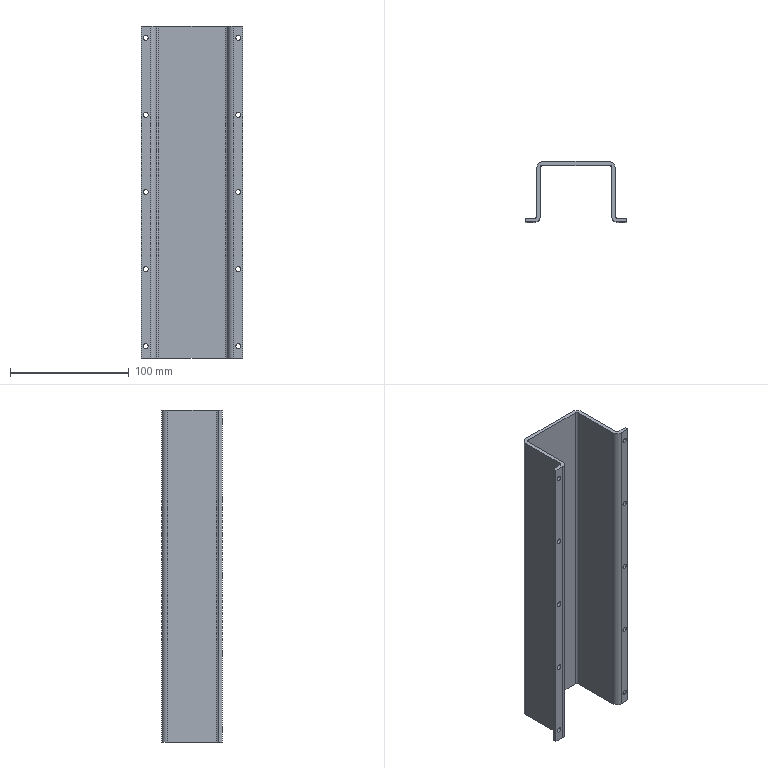Part | SolidWorks | features Extrusion 1, ICE 1, LPattern 1 | 1 solid | 42 faces | box 86 x 51 x 280 mm | volume 147456 mm3 | cylinder 28 | plane 14 | commonest cylinder face diameters 4 x24 10 x4
STEP:
#1=CARTESIAN_POINT('',(80.,3.,205.));
#2=VERTEX_POINT('',#1);
#3=CARTESIAN_POINT('',(84.,3.,205.));
#4=VERTEX_POINT('',#3);
#5=CARTESIAN_POINT('',(82.,3.,205.));
#6=DIRECTION('',(0.,-1.,0.));
#7=DIRECTION('',(1.,0.,0.));
#8=AXIS2_PLACEMENT_3D('',#5,#6,#7);
#9=CIRCLE('',#8,2.);
#10=EDGE_CURVE('',#2,#4,#9,.T.);
#11=ORIENTED_EDGE('',*,*,#10,.F.);
#12=CARTESIAN_POINT('',(80.,0.,205.));
#13=VERTEX_POINT('',#12);
#14=CARTESIAN_POINT('',(80.,10.,205.));
#15=DIRECTION('',(0.,-1.,0.));
#16=VECTOR('',#15,1000.);
#17=LINE('',#14,#16);
#18=EDGE_CURVE('',#2,#13,#17,.T.);
#19=ORIENTED_EDGE('',*,*,#18,.T.);
#20=CARTESIAN_POINT('',(84.,0.,205.));
#21=VERTEX_POINT('',#20);
#22=CARTESIAN_POINT('',(82.,0.,205.));
#23=DIRECTION('',(0.,-1.,0.));
#24=DIRECTION('',(1.,0.,0.));
#25=AXIS2_PLACEMENT_3D('',#22,#23,#24);
#26=CIRCLE('',#25,2.);
#27=EDGE_CURVE('',#13,#21,#26,.T.);
#28=ORIENTED_EDGE('',*,*,#27,.T.);
#29=CARTESIAN_POINT('',(84.,10.,205.));
#30=DIRECTION('',(0.,-1.,0.));
#31=VECTOR('',#30,1000.);
#32=LINE('',#29,#31);
#33=EDGE_CURVE('',#4,#21,#32,.T.);
#34=ORIENTED_EDGE('',*,*,#33,.F.);
#35=EDGE_LOOP('',(#11,#19,#28,#34));
#36=FACE_OUTER_BOUND('',#35,.T.);
#37=CARTESIAN_POINT('',(82.,10.,205.));
#38=DIRECTION('',(0.,-1.,0.));
#39=DIRECTION('',(1.,0.,0.));
#40=AXIS2_PLACEMENT_3D('',#37,#38,#39);
#41=CYLINDRICAL_SURFACE('',#40,2.);
#42=ADVANCED_FACE('',(#36),#41,.F.);
#43=CARTESIAN_POINT('',(80.,3.,140.));
#44=VERTEX_POINT('',#43);
#45=CARTESIAN_POINT('',(84.,3.,140.));
#46=VERTEX_POINT('',#45);
#47=CARTESIAN_POINT('',(82.,3.,140.));
#48=DIRECTION('',(0.,-1.,0.));
#49=DIRECTION('',(1.,0.,0.));
#50=AXIS2_PLACEMENT_3D('',#47,#48,#49);
#51=CIRCLE('',#50,2.);
#52=EDGE_CURVE('',#44,#46,#51,.T.);
#53=ORIENTED_EDGE('',*,*,#52,.F.);
#54=CARTESIAN_POINT('',(80.,0.,140.));
#55=VERTEX_POINT('',#54);
#56=CARTESIAN_POINT('',(80.,10.,140.));
#57=DIRECTION('',(0.,-1.,0.));
#58=VECTOR('',#57,1000.);
#59=LINE('',#56,#58);
#60=EDGE_CURVE('',#44,#55,#59,.T.);
#61=ORIENTED_EDGE('',*,*,#60,.T.);
#62=CARTESIAN_POINT('',(84.,0.,140.));
#63=VERTEX_POINT('',#62);
#64=CARTESIAN_POINT('',(82.,0.,140.));
#65=DIRECTION('',(0.,-1.,0.));
#66=DIRECTION('',(1.,0.,0.));
#67=AXIS2_PLACEMENT_3D('',#64,#65,#66);
#68=CIRCLE('',#67,2.);
#69=EDGE_CURVE('',#55,#63,#68,.T.);
#70=ORIENTED_EDGE('',*,*,#69,.T.);
#71=CARTESIAN_POINT('',(84.,10.,140.));
#72=DIRECTION('',(0.,-1.,0.));
#73=VECTOR('',#72,1000.);
#74=LINE('',#71,#73);
#75=EDGE_CURVE('',#46,#63,#74,.T.);
#76=ORIENTED_EDGE('',*,*,#75,.F.);
#77=EDGE_LOOP('',(#53,#61,#70,#76));
#78=FACE_OUTER_BOUND('',#77,.T.);
#79=CARTESIAN_POINT('',(82.,10.,140.));
#80=DIRECTION('',(0.,-1.,0.));
#81=DIRECTION('',(1.,0.,0.));
#82=AXIS2_PLACEMENT_3D('',#79,#80,#81);
#83=CYLINDRICAL_SURFACE('',#82,2.);
#84=ADVANCED_FACE('',(#78),#83,.F.);
#85=CARTESIAN_POINT('',(80.,3.,75.));
#86=VERTEX_POINT('',#85);
#87=CARTESIAN_POINT('',(84.,3.,75.));
#88=VERTEX_POINT('',#87);
#89=CARTESIAN_POINT('',(82.,3.,75.));
#90=DIRECTION('',(0.,-1.,0.));
#91=DIRECTION('',(1.,0.,0.));
#92=AXIS2_PLACEMENT_3D('',#89,#90,#91);
#93=CIRCLE('',#92,2.);
#94=EDGE_CURVE('',#86,#88,#93,.T.);
#95=ORIENTED_EDGE('',*,*,#94,.F.);
#96=CARTESIAN_POINT('',(80.,0.,75.));
#97=VERTEX_POINT('',#96);
#98=CARTESIAN_POINT('',(80.,10.,75.));
#99=DIRECTION('',(0.,-1.,0.));
#100=VECTOR('',#99,1000.);
#101=LINE('',#98,#100);
#102=EDGE_CURVE('',#86,#97,#101,.T.);
#103=ORIENTED_EDGE('',*,*,#102,.T.);
#104=CARTESIAN_POINT('',(84.,0.,75.));
#105=VERTEX_POINT('',#104);
#106=CARTESIAN_POINT('',(82.,0.,75.));
#107=DIRECTION('',(0.,-1.,0.));
#108=DIRECTION('',(1.,0.,0.));
#109=AXIS2_PLACEMENT_3D('',#106,#107,#108);
#110=CIRCLE('',#109,2.);
#111=EDGE_CURVE('',#97,#105,#110,.T.);
#112=ORIENTED_EDGE('',*,*,#111,.T.);
#113=CARTESIAN_POINT('',(84.,10.,75.));
#114=DIRECTION('',(0.,-1.,0.));
#115=VECTOR('',#114,1000.);
#116=LINE('',#113,#115);
#117=EDGE_CURVE('',#88,#105,#116,.T.);
#118=ORIENTED_EDGE('',*,*,#117,.F.);
#119=EDGE_LOOP('',(#95,#103,#112,#118));
#120=FACE_OUTER_BOUND('',#119,.T.);
#121=CARTESIAN_POINT('',(82.,10.,75.));
#122=DIRECTION('',(0.,-1.,0.));
#123=DIRECTION('',(1.,0.,0.));
#124=AXIS2_PLACEMENT_3D('',#121,#122,#123);
#125=CYLINDRICAL_SURFACE('',#124,2.);
#126=ADVANCED_FACE('',(#120),#125,.F.);
#127=CARTESIAN_POINT('',(80.,3.,10.));
#128=VERTEX_POINT('',#127);
#129=CARTESIAN_POINT('',(84.,3.,10.));
#130=VERTEX_POINT('',#129);
#131=CARTESIAN_POINT('',(82.,3.,10.));
#132=DIRECTION('',(0.,-1.,0.));
#133=DIRECTION('',(1.,0.,0.));
#134=AXIS2_PLACEMENT_3D('',#131,#132,#133);
#135=CIRCLE('',#134,2.);
#136=EDGE_CURVE('',#128,#130,#135,.T.);
#137=ORIENTED_EDGE('',*,*,#136,.F.);
#138=CARTESIAN_POINT('',(80.,0.,10.));
#139=VERTEX_POINT('',#138);
#140=CARTESIAN_POINT('',(80.,10.,10.));
#141=DIRECTION('',(0.,-1.,0.));
#142=VECTOR('',#141,1000.);
#143=LINE('',#140,#142);
#144=EDGE_CURVE('',#128,#139,#143,.T.);
#145=ORIENTED_EDGE('',*,*,#144,.T.);
#146=CARTESIAN_POINT('',(84.,0.,10.));
#147=VERTEX_POINT('',#146);
#148=CARTESIAN_POINT('',(82.,0.,10.));
#149=DIRECTION('',(0.,-1.,0.));
#150=DIRECTION('',(1.,0.,0.));
#151=AXIS2_PLACEMENT_3D('',#148,#149,#150);
#152=CIRCLE('',#151,2.);
#153=EDGE_CURVE('',#139,#147,#152,.T.);
#154=ORIENTED_EDGE('',*,*,#153,.T.);
#155=CARTESIAN_POINT('',(84.,10.,10.));
#156=DIRECTION('',(0.,-1.,0.));
#157=VECTOR('',#156,1000.);
#158=LINE('',#155,#157);
#159=EDGE_CURVE('',#130,#147,#158,.T.);
#160=ORIENTED_EDGE('',*,*,#159,.F.);
#161=EDGE_LOOP('',(#137,#145,#154,#160));
#162=FACE_OUTER_BOUND('',#161,.T.);
#163=CARTESIAN_POINT('',(82.,10.,10.));
#164=DIRECTION('',(0.,-1.,0.));
#165=DIRECTION('',(1.,0.,0.));
#166=AXIS2_PLACEMENT_3D('',#163,#164,#165);
#167=CYLINDRICAL_SURFACE('',#166,2.);
#168=ADVANCED_FACE('',(#162),#167,.F.);
#169=CARTESIAN_POINT('',(2.,3.,140.));
#170=VERTEX_POINT('',#169);
#171=CARTESIAN_POINT('',(6.,3.,140.));
#172=VERTEX_POINT('',#171);
#173=CARTESIAN_POINT('',(4.,3.,140.));
#174=DIRECTION('',(0.,-1.,0.));
#175=DIRECTION('',(0.,0.,-1.));
#176=AXIS2_PLACEMENT_3D('',#173,#174,#175);
#177=CIRCLE('',#176,2.);
#178=EDGE_CURVE('',#170,#172,#177,.T.);
#179=ORIENTED_EDGE('',*,*,#178,.F.);
#180=CARTESIAN_POINT('',(2.,0.,140.));
#181=VERTEX_POINT('',#180);
#182=CARTESIAN_POINT('',(2.,10.,140.));
#183=DIRECTION('',(0.,-1.,0.));
#184=VECTOR('',#183,1000.);
#185=LINE('',#182,#184);
#186=EDGE_CURVE('',#170,#181,#185,.T.);
#187=ORIENTED_EDGE('',*,*,#186,.T.);
#188=CARTESIAN_POINT('',(6.,0.,140.));
#189=VERTEX_POINT('',#188);
#190=CARTESIAN_POINT('',(4.,0.,140.));
#191=DIRECTION('',(0.,-1.,0.));
#192=DIRECTION('',(1.,0.,0.));
#193=AXIS2_PLACEMENT_3D('',#190,#191,#192);
#194=CIRCLE('',#193,2.);
#195=EDGE_CURVE('',#181,#189,#194,.T.);
#196=ORIENTED_EDGE('',*,*,#195,.T.);
#197=CARTESIAN_POINT('',(6.,10.,140.));
#198=DIRECTION('',(0.,-1.,0.));
#199=VECTOR('',#198,1000.);
#200=LINE('',#197,#199);
#201=EDGE_CURVE('',#172,#189,#200,.T.);
#202=ORIENTED_EDGE('',*,*,#201,.F.);
#203=EDGE_LOOP('',(#179,#187,#196,#202));
#204=FACE_OUTER_BOUND('',#203,.T.);
#205=CARTESIAN_POINT('',(4.,10.,140.));
#206=DIRECTION('',(0.,-1.,0.));
#207=DIRECTION('',(1.,0.,0.));
#208=AXIS2_PLACEMENT_3D('',#205,#206,#207);
#209=CYLINDRICAL_SURFACE('',#208,2.);
#210=ADVANCED_FACE('',(#204),#209,.F.);
#211=CARTESIAN_POINT('',(2.,3.,75.));
#212=VERTEX_POINT('',#211);
#213=CARTESIAN_POINT('',(6.,3.,75.));
#214=VERTEX_POINT('',#213);
#215=CARTESIAN_POINT('',(4.,3.,75.));
#216=DIRECTION('',(0.,-1.,0.));
#217=DIRECTION('',(0.,0.,-1.));
#218=AXIS2_PLACEMENT_3D('',#215,#216,#217);
#219=CIRCLE('',#218,2.);
#220=EDGE_CURVE('',#212,#214,#219,.T.);
#221=ORIENTED_EDGE('',*,*,#220,.F.);
#222=CARTESIAN_POINT('',(2.,0.,75.));
#223=VERTEX_POINT('',#222);
#224=CARTESIAN_POINT('',(2.,10.,75.));
#225=DIRECTION('',(0.,-1.,0.));
#226=VECTOR('',#225,1000.);
#227=LINE('',#224,#226);
#228=EDGE_CURVE('',#212,#223,#227,.T.);
#229=ORIENTED_EDGE('',*,*,#228,.T.);
#230=CARTESIAN_POINT('',(6.,0.,75.));
#231=VERTEX_POINT('',#230);
#232=CARTESIAN_POINT('',(4.,0.,75.));
#233=DIRECTION('',(0.,-1.,0.));
#234=DIRECTION('',(1.,0.,0.));
#235=AXIS2_PLACEMENT_3D('',#232,#233,#234);
#236=CIRCLE('',#235,2.);
#237=EDGE_CURVE('',#223,#231,#236,.T.);
#238=ORIENTED_EDGE('',*,*,#237,.T.);
#239=CARTESIAN_POINT('',(6.,10.,75.));
#240=DIRECTION('',(0.,-1.,0.));
#241=VECTOR('',#240,1000.);
#242=LINE('',#239,#241);
#243=EDGE_CURVE('',#214,#231,#242,.T.);
#244=ORIENTED_EDGE('',*,*,#243,.F.);
#245=EDGE_LOOP('',(#221,#229,#238,#244));
#246=FACE_OUTER_BOUND('',#245,.T.);
#247=CARTESIAN_POINT('',(4.,10.,75.));
#248=DIRECTION('',(0.,-1.,0.));
#249=DIRECTION('',(1.,0.,0.));
#250=AXIS2_PLACEMENT_3D('',#247,#248,#249);
#251=CYLINDRICAL_SURFACE('',#250,2.);
#252=ADVANCED_FACE('',(#246),#251,.F.);
#253=CARTESIAN_POINT('',(2.,3.,10.));
#254=VERTEX_POINT('',#253);
#255=CARTESIAN_POINT('',(6.,3.,10.));
#256=VERTEX_POINT('',#255);
#257=CARTESIAN_POINT('',(4.,3.,10.));
#258=DIRECTION('',(0.,-1.,0.));
#259=DIRECTION('',(0.,0.,-1.));
#260=AXIS2_PLACEMENT_3D('',#257,#258,#259);
#261=CIRCLE('',#260,2.);
#262=EDGE_CURVE('',#254,#256,#261,.T.);
#263=ORIENTED_EDGE('',*,*,#262,.F.);
#264=CARTESIAN_POINT('',(2.,0.,10.));
#265=VERTEX_POINT('',#264);
#266=CARTESIAN_POINT('',(2.,10.,10.));
#267=DIRECTION('',(0.,-1.,0.));
#268=VECTOR('',#267,1000.);
#269=LINE('',#266,#268);
#270=EDGE_CURVE('',#254,#265,#269,.T.);
#271=ORIENTED_EDGE('',*,*,#270,.T.);
#272=CARTESIAN_POINT('',(6.,0.,10.));
#273=VERTEX_POINT('',#272);
#274=CARTESIAN_POINT('',(4.,0.,10.));
#275=DIRECTION('',(0.,-1.,0.));
#276=DIRECTION('',(1.,0.,0.));
#277=AXIS2_PLACEMENT_3D('',#274,#275,#276);
#278=CIRCLE('',#277,2.);
#279=EDGE_CURVE('',#265,#273,#278,.T.);
#280=ORIENTED_EDGE('',*,*,#279,.T.);
#281=CARTESIAN_POINT('',(6.,10.,10.));
#282=DIRECTION('',(0.,-1.,0.));
#283=VECTOR('',#282,1000.);
#284=LINE('',#281,#283);
#285=EDGE_CURVE('',#256,#273,#284,.T.);
#286=ORIENTED_EDGE('',*,*,#285,.F.);
#287=EDGE_LOOP('',(#263,#271,#280,#286));
#288=FACE_OUTER_BOUND('',#287,.T.);
#289=CARTESIAN_POINT('',(4.,10.,10.));
#290=DIRECTION('',(0.,-1.,0.));
#291=DIRECTION('',(1.,0.,0.));
#292=AXIS2_PLACEMENT_3D('',#289,#290,#291);
#293=CYLINDRICAL_SURFACE('',#292,2.);
#294=ADVANCED_FACE('',(#288),#293,.F.);
#295=CARTESIAN_POINT('',(2.,3.,205.));
#296=VERTEX_POINT('',#295);
#297=CARTESIAN_POINT('',(6.,3.,205.));
#298=VERTEX_POINT('',#297);
#299=CARTESIAN_POINT('',(4.,3.,205.));
#300=DIRECTION('',(0.,-1.,0.));
#301=DIRECTION('',(0.,0.,-1.));
#302=AXIS2_PLACEMENT_3D('',#299,#300,#301);
#303=CIRCLE('',#302,2.);
#304=EDGE_CURVE('',#296,#298,#303,.T.);
#305=ORIENTED_EDGE('',*,*,#304,.F.);
#306=CARTESIAN_POINT('',(2.,0.,205.));
#307=VERTEX_POINT('',#306);
#308=CARTESIAN_POINT('',(2.,10.,205.));
#309=DIRECTION('',(0.,-1.,0.));
#310=VECTOR('',#309,1000.);
#311=LINE('',#308,#310);
#312=EDGE_CURVE('',#296,#307,#311,.T.);
#313=ORIENTED_EDGE('',*,*,#312,.T.);
#314=CARTESIAN_POINT('',(6.,0.,205.));
#315=VERTEX_POINT('',#314);
#316=CARTESIAN_POINT('',(4.,0.,205.));
#317=DIRECTION('',(0.,-1.,0.));
#318=DIRECTION('',(1.,0.,0.));
#319=AXIS2_PLACEMENT_3D('',#316,#317,#318);
#320=CIRCLE('',#319,2.);
#321=EDGE_CURVE('',#307,#315,#320,.T.);
#322=ORIENTED_EDGE('',*,*,#321,.T.);
#323=CARTESIAN_POINT('',(6.,10.,205.));
#324=DIRECTION('',(0.,-1.,0.));
#325=VECTOR('',#324,1000.);
#326=LINE('',#323,#325);
#327=EDGE_CURVE('',#298,#315,#326,.T.);
#328=ORIENTED_EDGE('',*,*,#327,.F.);
#329=EDGE_LOOP('',(#305,#313,#322,#328));
#330=FACE_OUTER_BOUND('',#329,.T.);
#331=CARTESIAN_POINT('',(4.,10.,205.));
#332=DIRECTION('',(0.,-1.,0.));
#333=DIRECTION('',(1.,0.,0.));
#334=AXIS2_PLACEMENT_3D('',#331,#332,#333);
#335=CYLINDRICAL_SURFACE('',#334,2.);
#336=ADVANCED_FACE('',(#330),#335,.F.);
#337=CARTESIAN_POINT('',(80.,3.,270.));
#338=VERTEX_POINT('',#337);
#339=CARTESIAN_POINT('',(84.,3.,270.));
#340=VERTEX_POINT('',#339);
#341=CARTESIAN_POINT('',(82.,3.,270.));
#342=DIRECTION('',(0.,-1.,0.));
#343=DIRECTION('',(1.,0.,0.));
#344=AXIS2_PLACEMENT_3D('',#341,#342,#343);
#345=CIRCLE('',#344,2.);
#346=EDGE_CURVE('',#338,#340,#345,.T.);
#347=ORIENTED_EDGE('',*,*,#346,.F.);
#348=CARTESIAN_POINT('',(80.,0.,270.));
#349=VERTEX_POINT('',#348);
#350=CARTESIAN_POINT('',(80.,10.,270.));
#351=DIRECTION('',(0.,-1.,0.));
#352=VECTOR('',#351,1000.);
#353=LINE('',#350,#352);
#354=EDGE_CURVE('',#338,#349,#353,.T.);
#355=ORIENTED_EDGE('',*,*,#354,.T.);
#356=CARTESIAN_POINT('',(84.,0.,270.));
#357=VERTEX_POINT('',#356);
#358=CARTESIAN_POINT('',(82.,0.,270.));
#359=DIRECTION('',(0.,-1.,0.));
#360=DIRECTION('',(1.,0.,0.));
#361=AXIS2_PLACEMENT_3D('',#358,#359,#360);
#362=CIRCLE('',#361,2.);
#363=EDGE_CURVE('',#349,#357,#362,.T.);
#364=ORIENTED_EDGE('',*,*,#363,.T.);
#365=CARTESIAN_POINT('',(84.,10.,270.));
#366=DIRECTION('',(0.,-1.,0.));
#367=VECTOR('',#366,1000.);
#368=LINE('',#365,#367);
#369=EDGE_CURVE('',#340,#357,#368,.T.);
#370=ORIENTED_EDGE('',*,*,#369,.F.);
#371=EDGE_LOOP('',(#347,#355,#364,#370));
#372=FACE_OUTER_BOUND('',#371,.T.);
#373=CARTESIAN_POINT('',(82.,10.,270.));
#374=DIRECTION('',(0.,-1.,0.));
#375=DIRECTION('',(1.,0.,0.));
#376=AXIS2_PLACEMENT_3D('',#373,#374,#375);
#377=CYLINDRICAL_SURFACE('',#376,2.);
#378=ADVANCED_FACE('',(#372),#377,.F.);
#379=CARTESIAN_POINT('',(2.,3.,270.));
#380=VERTEX_POINT('',#379);
#381=CARTESIAN_POINT('',(6.,3.,270.));
#382=VERTEX_POINT('',#381);
#383=CARTESIAN_POINT('',(4.,3.,270.));
#384=DIRECTION('',(0.,-1.,0.));
#385=DIRECTION('',(0.,0.,-1.));
#386=AXIS2_PLACEMENT_3D('',#383,#384,#385);
#387=CIRCLE('',#386,2.);
#388=EDGE_CURVE('',#380,#382,#387,.T.);
#389=ORIENTED_EDGE('',*,*,#388,.F.);
#390=CARTESIAN_POINT('',(2.,0.,270.));
#391=VERTEX_POINT('',#390);
#392=CARTESIAN_POINT('',(2.,10.,270.));
#393=DIRECTION('',(0.,-1.,0.));
#394=VECTOR('',#393,1000.);
#395=LINE('',#392,#394);
#396=EDGE_CURVE('',#380,#391,#395,.T.);
#397=ORIENTED_EDGE('',*,*,#396,.T.);
#398=CARTESIAN_POINT('',(6.,0.,270.));
#399=VERTEX_POINT('',#398);
#400=CARTESIAN_POINT('',(4.,0.,270.));
#401=DIRECTION('',(0.,-1.,0.));
#402=DIRECTION('',(1.,0.,0.));
#403=AXIS2_PLACEMENT_3D('',#400,#401,#402);
#404=CIRCLE('',#403,2.);
#405=EDGE_CURVE('',#391,#399,#404,.T.);
#406=ORIENTED_EDGE('',*,*,#405,.T.);
#407=CARTESIAN_POINT('',(6.,10.,270.));
#408=DIRECTION('',(0.,-1.,0.));
#409=VECTOR('',#408,1000.);
#410=LINE('',#407,#409);
#411=EDGE_CURVE('',#382,#399,#410,.T.);
#412=ORIENTED_EDGE('',*,*,#411,.F.);
#413=EDGE_LOOP('',(#389,#397,#406,#412));
#414=FACE_OUTER_BOUND('',#413,.T.);
#415=CARTESIAN_POINT('',(4.,10.,270.));
#416=DIRECTION('',(0.,-1.,0.));
#417=DIRECTION('',(1.,0.,0.));
#418=AXIS2_PLACEMENT_3D('',#415,#416,#417);
#419=CYLINDRICAL_SURFACE('',#418,2.);
#420=ADVANCED_FACE('',(#414),#419,.F.);
#421=CARTESIAN_POINT('',(4.,0.,140.));
#422=DIRECTION('',(0.,-1.,0.));
#423=DIRECTION('',(1.,0.,0.));
#424=AXIS2_PLACEMENT_3D('',#421,#422,#423);
#425=CIRCLE('',#424,2.);
#426=EDGE_CURVE('',#189,#181,#425,.T.);
#427=ORIENTED_EDGE('',*,*,#426,.F.);
#428=ORIENTED_EDGE('',*,*,#195,.F.);
#429=EDGE_LOOP('',(#427,#428));
#430=FACE_BOUND('',#429,.T.);
#431=CARTESIAN_POINT('',(4.,0.,75.));
#432=DIRECTION('',(0.,-1.,0.));
#433=DIRECTION('',(1.,0.,0.));
#434=AXIS2_PLACEMENT_3D('',#431,#432,#433);
#435=CIRCLE('',#434,2.);
#436=EDGE_CURVE('',#231,#223,#435,.T.);
#437=ORIENTED_EDGE('',*,*,#436,.F.);
#438=ORIENTED_EDGE('',*,*,#237,.F.);
#439=EDGE_LOOP('',(#437,#438));
#440=FACE_BOUND('',#439,.T.);
#441=CARTESIAN_POINT('',(4.,0.,10.));
#442=DIRECTION('',(0.,-1.,0.));
#443=DIRECTION('',(1.,0.,0.));
#444=AXIS2_PLACEMENT_3D('',#441,#442,#443);
#445=CIRCLE('',#444,2.);
#446=EDGE_CURVE('',#273,#265,#445,.T.);
#447=ORIENTED_EDGE('',*,*,#446,.F.);
#448=ORIENTED_EDGE('',*,*,#279,.F.);
#449=EDGE_LOOP('',(#447,#448));
#450=FACE_BOUND('',#449,.T.);
#451=CARTESIAN_POINT('',(4.,0.,205.));
#452=DIRECTION('',(0.,-1.,0.));
#453=DIRECTION('',(1.,0.,0.));
#454=AXIS2_PLACEMENT_3D('',#451,#452,#453);
#455=CIRCLE('',#454,2.);
#456=EDGE_CURVE('',#315,#307,#455,.T.);
#457=ORIENTED_EDGE('',*,*,#456,.F.);
#458=ORIENTED_EDGE('',*,*,#321,.F.);
#459=EDGE_LOOP('',(#457,#458));
#460=FACE_BOUND('',#459,.T.);
#461=CARTESIAN_POINT('',(4.,0.,270.));
#462=DIRECTION('',(0.,-1.,0.));
#463=DIRECTION('',(1.,0.,0.));
#464=AXIS2_PLACEMENT_3D('',#461,#462,#463);
#465=CIRCLE('',#464,2.);
#466=EDGE_CURVE('',#399,#391,#465,.T.);
#467=ORIENTED_EDGE('',*,*,#466,.F.);
#468=ORIENTED_EDGE('',*,*,#405,.F.);
#469=EDGE_LOOP('',(#467,#468));
#470=FACE_BOUND('',#469,.T.);
#471=CARTESIAN_POINT('',(0.,0.,0.));
#472=VERTEX_POINT('',#471);
#473=CARTESIAN_POINT('',(8.,0.,0.));
#474=VERTEX_POINT('',#473);
#475=CARTESIAN_POINT('',(8.,0.,0.));
#476=DIRECTION('',(1.,0.,0.));
#477=VECTOR('',#476,1000.);
#478=LINE('',#475,#477);
#479=EDGE_CURVE('',#472,#474,#478,.T.);
#480=ORIENTED_EDGE('',*,*,#479,.T.);
#481=CARTESIAN_POINT('',(8.,0.,280.));
#482=VERTEX_POINT('',#481);
#483=CARTESIAN_POINT('',(8.,0.,280.));
#484=DIRECTION('',(0.,0.,-1.));
#485=VECTOR('',#484,1000.);
#486=LINE('',#483,#485);
#487=EDGE_CURVE('',#482,#474,#486,.T.);
#488=ORIENTED_EDGE('',*,*,#487,.F.);
#489=CARTESIAN_POINT('',(0.,0.,280.));
#490=VERTEX_POINT('',#489);
#491=CARTESIAN_POINT('',(8.,0.,280.));
#492=DIRECTION('',(1.,0.,0.));
#493=VECTOR('',#492,1000.);
#494=LINE('',#491,#493);
#495=EDGE_CURVE('',#490,#482,#494,.T.);
#496=ORIENTED_EDGE('',*,*,#495,.F.);
#497=CARTESIAN_POINT('',(0.,0.,280.));
#498=DIRECTION('',(0.,0.,-1.));
#499=VECTOR('',#498,1000.);
#500=LINE('',#497,#499);
#501=EDGE_CURVE('',#490,#472,#500,.T.);
#502=ORIENTED_EDGE('',*,*,#501,.T.);
#503=EDGE_LOOP('',(#480,#488,#496,#502));
#504=FACE_OUTER_BOUND('',#503,.T.);
#505=CARTESIAN_POINT('',(8.,0.,280.));
#506=DIRECTION('',(0.,1.,0.));
#507=DIRECTION('',(-1.,0.,0.));
#508=AXIS2_PLACEMENT_3D('',#505,#506,#507);
#509=PLANE('',#508);
#510=ADVANCED_FACE('',(#430,#440,#450,#460,#470,#504),#509,.F.);
#511=CARTESIAN_POINT('',(13.,5.,0.));
#512=VERTEX_POINT('',#511);
#513=CARTESIAN_POINT('',(8.,5.,0.));
#514=DIRECTION('',(0.,0.,1.));
#515=DIRECTION('',(-1.,0.,0.));
#516=AXIS2_PLACEMENT_3D('',#513,#514,#515);
#517=CIRCLE('',#516,5.);
#518=EDGE_CURVE('',#474,#512,#517,.T.);
#519=ORIENTED_EDGE('',*,*,#518,.T.);
#520=CARTESIAN_POINT('',(13.,5.,280.));
#521=VERTEX_POINT('',#520);
#522=CARTESIAN_POINT('',(13.,5.,280.));
#523=DIRECTION('',(0.,0.,-1.));
#524=VECTOR('',#523,1000.);
#525=LINE('',#522,#524);
#526=EDGE_CURVE('',#521,#512,#525,.T.);
#527=ORIENTED_EDGE('',*,*,#526,.F.);
#528=CARTESIAN_POINT('',(8.,5.,280.));
#529=DIRECTION('',(0.,0.,1.));
#530=DIRECTION('',(-1.,0.,0.));
#531=AXIS2_PLACEMENT_3D('',#528,#529,#530);
#532=CIRCLE('',#531,5.);
#533=EDGE_CURVE('',#482,#521,#532,.T.);
#534=ORIENTED_EDGE('',*,*,#533,.F.);
#535=ORIENTED_EDGE('',*,*,#487,.T.);
#536=EDGE_LOOP('',(#519,#527,#534,#535));
#537=FACE_OUTER_BOUND('',#536,.T.);
#538=CARTESIAN_POINT('',(8.,5.,280.));
#539=DIRECTION('',(0.,0.,-1.));
#540=DIRECTION('',(-1.,0.,0.));
#541=AXIS2_PLACEMENT_3D('',#538,#539,#540);
#542=CYLINDRICAL_SURFACE('',#541,5.);
#543=ADVANCED_FACE('',(#537),#542,.T.);
#544=CARTESIAN_POINT('',(13.,46.,0.));
#545=VERTEX_POINT('',#544);
#546=CARTESIAN_POINT('',(13.,46.,0.));
#547=DIRECTION('',(0.,1.,0.));
#548=VECTOR('',#547,1000.);
#549=LINE('',#546,#548);
#550=EDGE_CURVE('',#512,#545,#549,.T.);
#551=ORIENTED_EDGE('',*,*,#550,.T.);
#552=CARTESIAN_POINT('',(13.,46.,280.));
#553=VERTEX_POINT('',#552);
#554=CARTESIAN_POINT('',(13.,46.,280.));
#555=DIRECTION('',(0.,0.,-1.));
#556=VECTOR('',#555,1000.);
#557=LINE('',#554,#556);
#558=EDGE_CURVE('',#553,#545,#557,.T.);
#559=ORIENTED_EDGE('',*,*,#558,.F.);
#560=CARTESIAN_POINT('',(13.,46.,280.));
#561=DIRECTION('',(0.,1.,0.));
#562=VECTOR('',#561,1000.);
#563=LINE('',#560,#562);
#564=EDGE_CURVE('',#521,#553,#563,.T.);
#565=ORIENTED_EDGE('',*,*,#564,.F.);
#566=ORIENTED_EDGE('',*,*,#526,.T.);
#567=EDGE_LOOP('',(#551,#559,#565,#566));
#568=FACE_OUTER_BOUND('',#567,.T.);
#569=CARTESIAN_POINT('',(13.,46.,280.));
#570=DIRECTION('',(-1.,0.,0.));
#571=DIRECTION('',(0.,0.,1.));
#572=AXIS2_PLACEMENT_3D('',#569,#570,#571);
#573=PLANE('',#572);
#574=ADVANCED_FACE('',(#568),#573,.F.);
#575=CARTESIAN_POINT('',(15.,48.,0.));
#576=VERTEX_POINT('',#575);
#577=CARTESIAN_POINT('',(15.,46.,0.));
#578=DIRECTION('',(0.,0.,-1.));
#579=DIRECTION('',(1.,0.,0.));
#580=AXIS2_PLACEMENT_3D('',#577,#578,#579);
#581=CIRCLE('',#580,2.);
#582=EDGE_CURVE('',#545,#576,#581,.T.);
#583=ORIENTED_EDGE('',*,*,#582,.T.);
#584=CARTESIAN_POINT('',(15.,48.,280.));
#585=VERTEX_POINT('',#584);
#586=CARTESIAN_POINT('',(15.,48.,280.));
#587=DIRECTION('',(0.,0.,-1.));
#588=VECTOR('',#587,1000.);
#589=LINE('',#586,#588);
#590=EDGE_CURVE('',#585,#576,#589,.T.);
#591=ORIENTED_EDGE('',*,*,#590,.F.);
#592=CARTESIAN_POINT('',(15.,46.,280.));
#593=DIRECTION('',(0.,0.,-1.));
#594=DIRECTION('',(1.,0.,0.));
#595=AXIS2_PLACEMENT_3D('',#592,#593,#594);
#596=CIRCLE('',#595,2.);
#597=EDGE_CURVE('',#553,#585,#596,.T.);
#598=ORIENTED_EDGE('',*,*,#597,.F.);
#599=ORIENTED_EDGE('',*,*,#558,.T.);
#600=EDGE_LOOP('',(#583,#591,#598,#599));
#601=FACE_OUTER_BOUND('',#600,.T.);
#602=CARTESIAN_POINT('',(15.,46.,280.));
#603=DIRECTION('',(0.,0.,-1.));
#604=DIRECTION('',(-1.,0.,0.));
#605=AXIS2_PLACEMENT_3D('',#602,#603,#604);
#606=CYLINDRICAL_SURFACE('',#605,2.);
#607=ADVANCED_FACE('',(#601),#606,.F.);
#608=CARTESIAN_POINT('',(71.,48.,0.));
#609=VERTEX_POINT('',#608);
#610=CARTESIAN_POINT('',(71.,48.,0.));
#611=DIRECTION('',(1.,0.,0.));
#612=VECTOR('',#611,1000.);
#613=LINE('',#610,#612);
#614=EDGE_CURVE('',#576,#609,#613,.T.);
#615=ORIENTED_EDGE('',*,*,#614,.T.);
#616=CARTESIAN_POINT('',(71.,48.,280.));
#617=VERTEX_POINT('',#616);
#618=CARTESIAN_POINT('',(71.,48.,280.));
#619=DIRECTION('',(0.,0.,-1.));
#620=VECTOR('',#619,1000.);
#621=LINE('',#618,#620);
#622=EDGE_CURVE('',#617,#609,#621,.T.);
#623=ORIENTED_EDGE('',*,*,#622,.F.);
#624=CARTESIAN_POINT('',(71.,48.,280.));
#625=DIRECTION('',(1.,0.,0.));
#626=VECTOR('',#625,1000.);
#627=LINE('',#624,#626);
#628=EDGE_CURVE('',#585,#617,#627,.T.);
#629=ORIENTED_EDGE('',*,*,#628,.F.);
#630=ORIENTED_EDGE('',*,*,#590,.T.);
#631=EDGE_LOOP('',(#615,#623,#629,#630));
#632=FACE_OUTER_BOUND('',#631,.T.);
#633=CARTESIAN_POINT('',(71.,48.,280.));
#634=DIRECTION('',(0.,1.,0.));
#635=DIRECTION('',(-1.,0.,0.));
#636=AXIS2_PLACEMENT_3D('',#633,#634,#635);
#637=PLANE('',#636);
#638=ADVANCED_FACE('',(#632),#637,.F.);
#639=CARTESIAN_POINT('',(73.,46.,0.));
#640=VERTEX_POINT('',#639);
#641=CARTESIAN_POINT('',(71.,46.,0.));
#642=DIRECTION('',(0.,0.,-1.));
#643=DIRECTION('',(1.,0.,0.));
#644=AXIS2_PLACEMENT_3D('',#641,#642,#643);
#645=CIRCLE('',#644,2.);
#646=EDGE_CURVE('',#609,#640,#645,.T.);
#647=ORIENTED_EDGE('',*,*,#646,.T.);
#648=CARTESIAN_POINT('',(73.,46.,280.));
#649=VERTEX_POINT('',#648);
#650=CARTESIAN_POINT('',(73.,46.,280.));
#651=DIRECTION('',(0.,0.,-1.));
#652=VECTOR('',#651,1000.);
#653=LINE('',#650,#652);
#654=EDGE_CURVE('',#649,#640,#653,.T.);
#655=ORIENTED_EDGE('',*,*,#654,.F.);
#656=CARTESIAN_POINT('',(71.,46.,280.));
#657=DIRECTION('',(0.,0.,-1.));
#658=DIRECTION('',(1.,0.,0.));
#659=AXIS2_PLACEMENT_3D('',#656,#657,#658);
#660=CIRCLE('',#659,2.);
#661=EDGE_CURVE('',#617,#649,#660,.T.);
#662=ORIENTED_EDGE('',*,*,#661,.F.);
#663=ORIENTED_EDGE('',*,*,#622,.T.);
#664=EDGE_LOOP('',(#647,#655,#662,#663));
#665=FACE_OUTER_BOUND('',#664,.T.);
#666=CARTESIAN_POINT('',(71.,46.,280.));
#667=DIRECTION('',(0.,0.,-1.));
#668=DIRECTION('',(-1.,0.,0.));
#669=AXIS2_PLACEMENT_3D('',#666,#667,#668);
#670=CYLINDRICAL_SURFACE('',#669,2.);
#671=ADVANCED_FACE('',(#665),#670,.F.);
#672=CARTESIAN_POINT('',(73.,5.,0.));
#673=VERTEX_POINT('',#672);
#674=CARTESIAN_POINT('',(73.,5.,0.));
#675=DIRECTION('',(0.,-1.,0.));
#676=VECTOR('',#675,1000.);
#677=LINE('',#674,#676);
#678=EDGE_CURVE('',#640,#673,#677,.T.);
#679=ORIENTED_EDGE('',*,*,#678,.T.);
#680=CARTESIAN_POINT('',(73.,5.,280.));
#681=VERTEX_POINT('',#680);
#682=CARTESIAN_POINT('',(73.,5.,280.));
#683=DIRECTION('',(0.,0.,-1.));
#684=VECTOR('',#683,1000.);
#685=LINE('',#682,#684);
#686=EDGE_CURVE('',#681,#673,#685,.T.);
#687=ORIENTED_EDGE('',*,*,#686,.F.);
#688=CARTESIAN_POINT('',(73.,5.,280.));
#689=DIRECTION('',(0.,-1.,0.));
#690=VECTOR('',#689,1000.);
#691=LINE('',#688,#690);
#692=EDGE_CURVE('',#649,#681,#691,.T.);
#693=ORIENTED_EDGE('',*,*,#692,.F.);
#694=ORIENTED_EDGE('',*,*,#654,.T.);
#695=EDGE_LOOP('',(#679,#687,#693,#694));
#696=FACE_OUTER_BOUND('',#695,.T.);
#697=CARTESIAN_POINT('',(73.,5.,280.));
#698=DIRECTION('',(1.,0.,0.));
#699=DIRECTION('',(0.,0.,-1.));
#700=AXIS2_PLACEMENT_3D('',#697,#698,#699);
#701=PLANE('',#700);
#702=ADVANCED_FACE('',(#696),#701,.F.);
#703=CARTESIAN_POINT('',(78.,0.,0.));
#704=VERTEX_POINT('',#703);
#705=CARTESIAN_POINT('',(78.,5.,0.));
#706=DIRECTION('',(0.,0.,1.));
#707=DIRECTION('',(-1.,0.,0.));
#708=AXIS2_PLACEMENT_3D('',#705,#706,#707);
#709=CIRCLE('',#708,5.);
#710=EDGE_CURVE('',#673,#704,#709,.T.);
#711=ORIENTED_EDGE('',*,*,#710,.T.);
#712=CARTESIAN_POINT('',(78.,0.,280.));
#713=VERTEX_POINT('',#712);
#714=CARTESIAN_POINT('',(78.,0.,280.));
#715=DIRECTION('',(0.,0.,-1.));
#716=VECTOR('',#715,1000.);
#717=LINE('',#714,#716);
#718=EDGE_CURVE('',#713,#704,#717,.T.);
#719=ORIENTED_EDGE('',*,*,#718,.F.);
#720=CARTESIAN_POINT('',(78.,5.,280.));
#721=DIRECTION('',(0.,0.,1.));
#722=DIRECTION('',(-1.,0.,0.));
#723=AXIS2_PLACEMENT_3D('',#720,#721,#722);
#724=CIRCLE('',#723,5.);
#725=EDGE_CURVE('',#681,#713,#724,.T.);
#726=ORIENTED_EDGE('',*,*,#725,.F.);
#727=ORIENTED_EDGE('',*,*,#686,.T.);
#728=EDGE_LOOP('',(#711,#719,#726,#727));
#729=FACE_OUTER_BOUND('',#728,.T.);
#730=CARTESIAN_POINT('',(78.,5.,280.));
#731=DIRECTION('',(0.,0.,-1.));
#732=DIRECTION('',(-1.,0.,0.));
#733=AXIS2_PLACEMENT_3D('',#730,#731,#732);
#734=CYLINDRICAL_SURFACE('',#733,5.);
#735=ADVANCED_FACE('',(#729),#734,.T.);
#736=CARTESIAN_POINT('',(82.,0.,205.));
#737=DIRECTION('',(0.,-1.,0.));
#738=DIRECTION('',(1.,0.,0.));
#739=AXIS2_PLACEMENT_3D('',#736,#737,#738);
#740=CIRCLE('',#739,2.);
#741=EDGE_CURVE('',#21,#13,#740,.T.);
#742=ORIENTED_EDGE('',*,*,#741,.F.);
#743=ORIENTED_EDGE('',*,*,#27,.F.);
#744=EDGE_LOOP('',(#742,#743));
#745=FACE_BOUND('',#744,.T.);
#746=CARTESIAN_POINT('',(82.,0.,140.));
#747=DIRECTION('',(0.,-1.,0.));
#748=DIRECTION('',(1.,0.,0.));
#749=AXIS2_PLACEMENT_3D('',#746,#747,#748);
#750=CIRCLE('',#749,2.);
#751=EDGE_CURVE('',#63,#55,#750,.T.);
#752=ORIENTED_EDGE('',*,*,#751,.F.);
#753=ORIENTED_EDGE('',*,*,#69,.F.);
#754=EDGE_LOOP('',(#752,#753));
#755=FACE_BOUND('',#754,.T.);
#756=CARTESIAN_POINT('',(82.,0.,75.));
#757=DIRECTION('',(0.,-1.,0.));
#758=DIRECTION('',(1.,0.,0.));
#759=AXIS2_PLACEMENT_3D('',#756,#757,#758);
#760=CIRCLE('',#759,2.);
#761=EDGE_CURVE('',#105,#97,#760,.T.);
#762=ORIENTED_EDGE('',*,*,#761,.F.);
#763=ORIENTED_EDGE('',*,*,#111,.F.);
#764=EDGE_LOOP('',(#762,#763));
#765=FACE_BOUND('',#764,.T.);
#766=CARTESIAN_POINT('',(82.,0.,10.));
#767=DIRECTION('',(0.,-1.,0.));
#768=DIRECTION('',(1.,0.,0.));
#769=AXIS2_PLACEMENT_3D('',#766,#767,#768);
#770=CIRCLE('',#769,2.);
#771=EDGE_CURVE('',#147,#139,#770,.T.);
#772=ORIENTED_EDGE('',*,*,#771,.F.);
#773=ORIENTED_EDGE('',*,*,#153,.F.);
#774=EDGE_LOOP('',(#772,#773));
#775=FACE_BOUND('',#774,.T.);
#776=CARTESIAN_POINT('',(82.,0.,270.));
#777=DIRECTION('',(0.,-1.,0.));
#778=DIRECTION('',(1.,0.,0.));
#779=AXIS2_PLACEMENT_3D('',#776,#777,#778);
#780=CIRCLE('',#779,2.);
#781=EDGE_CURVE('',#357,#349,#780,.T.);
#782=ORIENTED_EDGE('',*,*,#781,.F.);
#783=ORIENTED_EDGE('',*,*,#363,.F.);
#784=EDGE_LOOP('',(#782,#783));
#785=FACE_BOUND('',#784,.T.);
#786=CARTESIAN_POINT('',(86.,0.,0.));
#787=VERTEX_POINT('',#786);
#788=CARTESIAN_POINT('',(86.,0.,0.));
#789=DIRECTION('',(1.,0.,0.));
#790=VECTOR('',#789,1000.);
#791=LINE('',#788,#790);
#792=EDGE_CURVE('',#704,#787,#791,.T.);
#793=ORIENTED_EDGE('',*,*,#792,.T.);
#794=CARTESIAN_POINT('',(86.,0.,280.));
#795=VERTEX_POINT('',#794);
#796=CARTESIAN_POINT('',(86.,0.,280.));
#797=DIRECTION('',(0.,0.,-1.));
#798=VECTOR('',#797,1000.);
#799=LINE('',#796,#798);
#800=EDGE_CURVE('',#795,#787,#799,.T.);
#801=ORIENTED_EDGE('',*,*,#800,.F.);
#802=CARTESIAN_POINT('',(86.,0.,280.));
#803=DIRECTION('',(1.,0.,0.));
#804=VECTOR('',#803,1000.);
#805=LINE('',#802,#804);
#806=EDGE_CURVE('',#713,#795,#805,.T.);
#807=ORIENTED_EDGE('',*,*,#806,.F.);
#808=ORIENTED_EDGE('',*,*,#718,.T.);
#809=EDGE_LOOP('',(#793,#801,#807,#808));
#810=FACE_OUTER_BOUND('',#809,.T.);
#811=CARTESIAN_POINT('',(86.,0.,280.));
#812=DIRECTION('',(0.,1.,0.));
#813=DIRECTION('',(0.,0.,1.));
#814=AXIS2_PLACEMENT_3D('',#811,#812,#813);
#815=PLANE('',#814);
#816=ADVANCED_FACE('',(#745,#755,#765,#775,#785,#810),#815,.F.);
#817=CARTESIAN_POINT('',(86.,3.,0.));
#818=VERTEX_POINT('',#817);
#819=CARTESIAN_POINT('',(86.,0.,0.));
#820=DIRECTION('',(0.,1.,0.));
#821=VECTOR('',#820,1000.);
#822=LINE('',#819,#821);
#823=EDGE_CURVE('',#787,#818,#822,.T.);
#824=ORIENTED_EDGE('',*,*,#823,.T.);
#825=CARTESIAN_POINT('',(86.,3.,280.));
#826=VERTEX_POINT('',#825);
#827=CARTESIAN_POINT('',(86.,3.,280.));
#828=DIRECTION('',(0.,0.,-1.));
#829=VECTOR('',#828,1000.);
#830=LINE('',#827,#829);
#831=EDGE_CURVE('',#826,#818,#830,.T.);
#832=ORIENTED_EDGE('',*,*,#831,.F.);
#833=CARTESIAN_POINT('',(86.,0.,280.));
#834=DIRECTION('',(0.,1.,0.));
#835=VECTOR('',#834,1000.);
#836=LINE('',#833,#835);
#837=EDGE_CURVE('',#795,#826,#836,.T.);
#838=ORIENTED_EDGE('',*,*,#837,.F.);
#839=ORIENTED_EDGE('',*,*,#800,.T.);
#840=EDGE_LOOP('',(#824,#832,#838,#839));
#841=FACE_OUTER_BOUND('',#840,.T.);
#842=CARTESIAN_POINT('',(86.,0.,280.));
#843=DIRECTION('',(-1.,0.,0.));
#844=DIRECTION('',(0.,-1.,0.));
#845=AXIS2_PLACEMENT_3D('',#842,#843,#844);
#846=PLANE('',#845);
#847=ADVANCED_FACE('',(#841),#846,.F.);
#848=CARTESIAN_POINT('',(82.,3.,205.));
#849=DIRECTION('',(0.,-1.,0.));
#850=DIRECTION('',(1.,0.,0.));
#851=AXIS2_PLACEMENT_3D('',#848,#849,#850);
#852=CIRCLE('',#851,2.);
#853=EDGE_CURVE('',#4,#2,#852,.T.);
#854=ORIENTED_EDGE('',*,*,#853,.T.);
#855=ORIENTED_EDGE('',*,*,#10,.T.);
#856=EDGE_LOOP('',(#854,#855));
#857=FACE_BOUND('',#856,.T.);
#858=CARTESIAN_POINT('',(82.,3.,140.));
#859=DIRECTION('',(0.,-1.,0.));
#860=DIRECTION('',(1.,0.,0.));
#861=AXIS2_PLACEMENT_3D('',#858,#859,#860);
#862=CIRCLE('',#861,2.);
#863=EDGE_CURVE('',#46,#44,#862,.T.);
#864=ORIENTED_EDGE('',*,*,#863,.T.);
#865=ORIENTED_EDGE('',*,*,#52,.T.);
#866=EDGE_LOOP('',(#864,#865));
#867=FACE_BOUND('',#866,.T.);
#868=CARTESIAN_POINT('',(82.,3.,75.));
#869=DIRECTION('',(0.,-1.,0.));
#870=DIRECTION('',(1.,0.,0.));
#871=AXIS2_PLACEMENT_3D('',#868,#869,#870);
#872=CIRCLE('',#871,2.);
#873=EDGE_CURVE('',#88,#86,#872,.T.);
#874=ORIENTED_EDGE('',*,*,#873,.T.);
#875=ORIENTED_EDGE('',*,*,#94,.T.);
#876=EDGE_LOOP('',(#874,#875));
#877=FACE_BOUND('',#876,.T.);
#878=CARTESIAN_POINT('',(82.,3.,10.));
#879=DIRECTION('',(0.,-1.,0.));
#880=DIRECTION('',(1.,0.,0.));
#881=AXIS2_PLACEMENT_3D('',#878,#879,#880);
#882=CIRCLE('',#881,2.);
#883=EDGE_CURVE('',#130,#128,#882,.T.);
#884=ORIENTED_EDGE('',*,*,#883,.T.);
#885=ORIENTED_EDGE('',*,*,#136,.T.);
#886=EDGE_LOOP('',(#884,#885));
#887=FACE_BOUND('',#886,.T.);
#888=CARTESIAN_POINT('',(82.,3.,270.));
#889=DIRECTION('',(0.,-1.,0.));
#890=DIRECTION('',(1.,0.,0.));
#891=AXIS2_PLACEMENT_3D('',#888,#889,#890);
#892=CIRCLE('',#891,2.);
#893=EDGE_CURVE('',#340,#338,#892,.T.);
#894=ORIENTED_EDGE('',*,*,#893,.T.);
#895=ORIENTED_EDGE('',*,*,#346,.T.);
#896=EDGE_LOOP('',(#894,#895));
#897=FACE_BOUND('',#896,.T.);
#898=CARTESIAN_POINT('',(78.,3.,0.));
#899=VERTEX_POINT('',#898);
#900=CARTESIAN_POINT('',(86.,3.,0.));
#901=DIRECTION('',(-1.,0.,0.));
#902=VECTOR('',#901,1000.);
#903=LINE('',#900,#902);
#904=EDGE_CURVE('',#818,#899,#903,.T.);
#905=ORIENTED_EDGE('',*,*,#904,.T.);
#906=CARTESIAN_POINT('',(78.,3.,280.));
#907=VERTEX_POINT('',#906);
#908=CARTESIAN_POINT('',(78.,3.,280.));
#909=DIRECTION('',(0.,0.,-1.));
#910=VECTOR('',#909,1000.);
#911=LINE('',#908,#910);
#912=EDGE_CURVE('',#907,#899,#911,.T.);
#913=ORIENTED_EDGE('',*,*,#912,.F.);
#914=CARTESIAN_POINT('',(86.,3.,280.));
#915=DIRECTION('',(-1.,0.,0.));
#916=VECTOR('',#915,1000.);
#917=LINE('',#914,#916);
#918=EDGE_CURVE('',#826,#907,#917,.T.);
#919=ORIENTED_EDGE('',*,*,#918,.F.);
#920=ORIENTED_EDGE('',*,*,#831,.T.);
#921=EDGE_LOOP('',(#905,#913,#919,#920));
#922=FACE_OUTER_BOUND('',#921,.T.);
#923=CARTESIAN_POINT('',(86.,3.,280.));
#924=DIRECTION('',(0.,-1.,0.));
#925=DIRECTION('',(1.,0.,0.));
#926=AXIS2_PLACEMENT_3D('',#923,#924,#925);
#927=PLANE('',#926);
#928=ADVANCED_FACE('',(#857,#867,#877,#887,#897,#922),#927,.F.);
#929=CARTESIAN_POINT('',(76.,5.,0.));
#930=VERTEX_POINT('',#929);
#931=CARTESIAN_POINT('',(78.,5.,0.));
#932=DIRECTION('',(0.,0.,-1.));
#933=DIRECTION('',(-1.,0.,0.));
#934=AXIS2_PLACEMENT_3D('',#931,#932,#933);
#935=CIRCLE('',#934,2.);
#936=EDGE_CURVE('',#899,#930,#935,.T.);
#937=ORIENTED_EDGE('',*,*,#936,.T.);
#938=CARTESIAN_POINT('',(76.,5.,280.));
#939=VERTEX_POINT('',#938);
#940=CARTESIAN_POINT('',(76.,5.,280.));
#941=DIRECTION('',(0.,0.,-1.));
#942=VECTOR('',#941,1000.);
#943=LINE('',#940,#942);
#944=EDGE_CURVE('',#939,#930,#943,.T.);
#945=ORIENTED_EDGE('',*,*,#944,.F.);
#946=CARTESIAN_POINT('',(78.,5.,280.));
#947=DIRECTION('',(0.,0.,-1.));
#948=DIRECTION('',(-1.,0.,0.));
#949=AXIS2_PLACEMENT_3D('',#946,#947,#948);
#950=CIRCLE('',#949,2.);
#951=EDGE_CURVE('',#907,#939,#950,.T.);
#952=ORIENTED_EDGE('',*,*,#951,.F.);
#953=ORIENTED_EDGE('',*,*,#912,.T.);
#954=EDGE_LOOP('',(#937,#945,#952,#953));
#955=FACE_OUTER_BOUND('',#954,.T.);
#956=CARTESIAN_POINT('',(78.,5.,280.));
#957=DIRECTION('',(0.,0.,-1.));
#958=DIRECTION('',(-1.,0.,0.));
#959=AXIS2_PLACEMENT_3D('',#956,#957,#958);
#960=CYLINDRICAL_SURFACE('',#959,2.);
#961=ADVANCED_FACE('',(#955),#960,.F.);
#962=CARTESIAN_POINT('',(76.,46.,0.));
#963=VERTEX_POINT('',#962);
#964=CARTESIAN_POINT('',(76.,5.,0.));
#965=DIRECTION('',(0.,1.,0.));
#966=VECTOR('',#965,1000.);
#967=LINE('',#964,#966);
#968=EDGE_CURVE('',#930,#963,#967,.T.);
#969=ORIENTED_EDGE('',*,*,#968,.T.);
#970=CARTESIAN_POINT('',(76.,46.,280.));
#971=VERTEX_POINT('',#970);
#972=CARTESIAN_POINT('',(76.,46.,280.));
#973=DIRECTION('',(0.,0.,-1.));
#974=VECTOR('',#973,1000.);
#975=LINE('',#972,#974);
#976=EDGE_CURVE('',#971,#963,#975,.T.);
#977=ORIENTED_EDGE('',*,*,#976,.F.);
#978=CARTESIAN_POINT('',(76.,5.,280.));
#979=DIRECTION('',(0.,1.,0.));
#980=VECTOR('',#979,1000.);
#981=LINE('',#978,#980);
#982=EDGE_CURVE('',#939,#971,#981,.T.);
#983=ORIENTED_EDGE('',*,*,#982,.F.);
#984=ORIENTED_EDGE('',*,*,#944,.T.);
#985=EDGE_LOOP('',(#969,#977,#983,#984));
#986=FACE_OUTER_BOUND('',#985,.T.);
#987=CARTESIAN_POINT('',(76.,5.,280.));
#988=DIRECTION('',(-1.,0.,0.));
#989=DIRECTION('',(0.,-1.,0.));
#990=AXIS2_PLACEMENT_3D('',#987,#988,#989);
#991=PLANE('',#990);
#992=ADVANCED_FACE('',(#986),#991,.F.);
#993=CARTESIAN_POINT('',(71.,51.,0.));
#994=VERTEX_POINT('',#993);
#995=CARTESIAN_POINT('',(71.,46.,0.));
#996=DIRECTION('',(0.,0.,1.));
#997=DIRECTION('',(1.,0.,0.));
#998=AXIS2_PLACEMENT_3D('',#995,#996,#997);
#999=CIRCLE('',#998,5.);
#1000=EDGE_CURVE('',#963,#994,#999,.T.);
#1001=ORIENTED_EDGE('',*,*,#1000,.T.);
#1002=CARTESIAN_POINT('',(71.,51.,280.));
#1003=VERTEX_POINT('',#1002);
#1004=CARTESIAN_POINT('',(71.,51.,280.));
#1005=DIRECTION('',(0.,0.,-1.));
#1006=VECTOR('',#1005,1000.);
#1007=LINE('',#1004,#1006);
#1008=EDGE_CURVE('',#1003,#994,#1007,.T.);
#1009=ORIENTED_EDGE('',*,*,#1008,.F.);
#1010=CARTESIAN_POINT('',(71.,46.,280.));
#1011=DIRECTION('',(0.,0.,1.));
#1012=DIRECTION('',(1.,0.,0.));
#1013=AXIS2_PLACEMENT_3D('',#1010,#1011,#1012);
#1014=CIRCLE('',#1013,5.);
#1015=EDGE_CURVE('',#971,#1003,#1014,.T.);
#1016=ORIENTED_EDGE('',*,*,#1015,.F.);
#1017=ORIENTED_EDGE('',*,*,#976,.T.);
#1018=EDGE_LOOP('',(#1001,#1009,#1016,#1017));
#1019=FACE_OUTER_BOUND('',#1018,.T.);
#1020=CARTESIAN_POINT('',(71.,46.,280.));
#1021=DIRECTION('',(0.,0.,-1.));
#1022=DIRECTION('',(-1.,0.,0.));
#1023=AXIS2_PLACEMENT_3D('',#1020,#1021,#1022);
#1024=CYLINDRICAL_SURFACE('',#1023,5.);
#1025=ADVANCED_FACE('',(#1019),#1024,.T.);
#1026=CARTESIAN_POINT('',(15.,51.,0.));
#1027=VERTEX_POINT('',#1026);
#1028=CARTESIAN_POINT('',(71.,51.,0.));
#1029=DIRECTION('',(-1.,0.,0.));
#1030=VECTOR('',#1029,1000.);
#1031=LINE('',#1028,#1030);
#1032=EDGE_CURVE('',#994,#1027,#1031,.T.);
#1033=ORIENTED_EDGE('',*,*,#1032,.T.);
#1034=CARTESIAN_POINT('',(15.,51.,280.));
#1035=VERTEX_POINT('',#1034);
#1036=CARTESIAN_POINT('',(15.,51.,280.));
#1037=DIRECTION('',(0.,0.,-1.));
#1038=VECTOR('',#1037,1000.);
#1039=LINE('',#1036,#1038);
#1040=EDGE_CURVE('',#1035,#1027,#1039,.T.);
#1041=ORIENTED_EDGE('',*,*,#1040,.F.);
#1042=CARTESIAN_POINT('',(71.,51.,280.));
#1043=DIRECTION('',(-1.,0.,0.));
#1044=VECTOR('',#1043,1000.);
#1045=LINE('',#1042,#1044);
#1046=EDGE_CURVE('',#1003,#1035,#1045,.T.);
#1047=ORIENTED_EDGE('',*,*,#1046,.F.);
#1048=ORIENTED_EDGE('',*,*,#1008,.T.);
#1049=EDGE_LOOP('',(#1033,#1041,#1047,#1048));
#1050=FACE_OUTER_BOUND('',#1049,.T.);
#1051=CARTESIAN_POINT('',(71.,51.,280.));
#1052=DIRECTION('',(0.,-1.,0.));
#1053=DIRECTION('',(1.,0.,0.));
#1054=AXIS2_PLACEMENT_3D('',#1051,#1052,#1053);
#1055=PLANE('',#1054);
#1056=ADVANCED_FACE('',(#1050),#1055,.F.);
#1057=CARTESIAN_POINT('',(10.,46.,0.));
#1058=VERTEX_POINT('',#1057);
#1059=CARTESIAN_POINT('',(15.,46.,0.));
#1060=DIRECTION('',(0.,0.,1.));
#1061=DIRECTION('',(1.,0.,0.));
#1062=AXIS2_PLACEMENT_3D('',#1059,#1060,#1061);
#1063=CIRCLE('',#1062,5.);
#1064=EDGE_CURVE('',#1027,#1058,#1063,.T.);
#1065=ORIENTED_EDGE('',*,*,#1064,.T.);
#1066=CARTESIAN_POINT('',(10.,46.,280.));
#1067=VERTEX_POINT('',#1066);
#1068=CARTESIAN_POINT('',(10.,46.,280.));
#1069=DIRECTION('',(0.,0.,-1.));
#1070=VECTOR('',#1069,1000.);
#1071=LINE('',#1068,#1070);
#1072=EDGE_CURVE('',#1067,#1058,#1071,.T.);
#1073=ORIENTED_EDGE('',*,*,#1072,.F.);
#1074=CARTESIAN_POINT('',(15.,46.,280.));
#1075=DIRECTION('',(0.,0.,1.));
#1076=DIRECTION('',(1.,0.,0.));
#1077=AXIS2_PLACEMENT_3D('',#1074,#1075,#1076);
#1078=CIRCLE('',#1077,5.);
#1079=EDGE_CURVE('',#1035,#1067,#1078,.T.);
#1080=ORIENTED_EDGE('',*,*,#1079,.F.);
#1081=ORIENTED_EDGE('',*,*,#1040,.T.);
#1082=EDGE_LOOP('',(#1065,#1073,#1080,#1081));
#1083=FACE_OUTER_BOUND('',#1082,.T.);
#1084=CARTESIAN_POINT('',(15.,46.,280.));
#1085=DIRECTION('',(0.,0.,-1.));
#1086=DIRECTION('',(-1.,0.,0.));
#1087=AXIS2_PLACEMENT_3D('',#1084,#1085,#1086);
#1088=CYLINDRICAL_SURFACE('',#1087,5.);
#1089=ADVANCED_FACE('',(#1083),#1088,.T.);
#1090=CARTESIAN_POINT('',(10.,5.,0.));
#1091=VERTEX_POINT('',#1090);
#1092=CARTESIAN_POINT('',(10.,46.,0.));
#1093=DIRECTION('',(0.,-1.,0.));
#1094=VECTOR('',#1093,1000.);
#1095=LINE('',#1092,#1094);
#1096=EDGE_CURVE('',#1058,#1091,#1095,.T.);
#1097=ORIENTED_EDGE('',*,*,#1096,.T.);
#1098=CARTESIAN_POINT('',(10.,5.,280.));
#1099=VERTEX_POINT('',#1098);
#1100=CARTESIAN_POINT('',(10.,5.,280.));
#1101=DIRECTION('',(0.,0.,-1.));
#1102=VECTOR('',#1101,1000.);
#1103=LINE('',#1100,#1102);
#1104=EDGE_CURVE('',#1099,#1091,#1103,.T.);
#1105=ORIENTED_EDGE('',*,*,#1104,.F.);
#1106=CARTESIAN_POINT('',(10.,46.,280.));
#1107=DIRECTION('',(0.,-1.,0.));
#1108=VECTOR('',#1107,1000.);
#1109=LINE('',#1106,#1108);
#1110=EDGE_CURVE('',#1067,#1099,#1109,.T.);
#1111=ORIENTED_EDGE('',*,*,#1110,.F.);
#1112=ORIENTED_EDGE('',*,*,#1072,.T.);
#1113=EDGE_LOOP('',(#1097,#1105,#1111,#1112));
#1114=FACE_OUTER_BOUND('',#1113,.T.);
#1115=CARTESIAN_POINT('',(10.,46.,280.));
#1116=DIRECTION('',(1.,0.,0.));
#1117=DIRECTION('',(0.,1.,0.));
#1118=AXIS2_PLACEMENT_3D('',#1115,#1116,#1117);
#1119=PLANE('',#1118);
#1120=ADVANCED_FACE('',(#1114),#1119,.F.);
#1121=CARTESIAN_POINT('',(8.,3.,0.));
#1122=VERTEX_POINT('',#1121);
#1123=CARTESIAN_POINT('',(8.,5.,0.));
#1124=DIRECTION('',(0.,0.,-1.));
#1125=DIRECTION('',(-1.,0.,0.));
#1126=AXIS2_PLACEMENT_3D('',#1123,#1124,#1125);
#1127=CIRCLE('',#1126,2.);
#1128=EDGE_CURVE('',#1091,#1122,#1127,.T.);
#1129=ORIENTED_EDGE('',*,*,#1128,.T.);
#1130=CARTESIAN_POINT('',(8.,3.,280.));
#1131=VERTEX_POINT('',#1130);
#1132=CARTESIAN_POINT('',(8.,3.,280.));
#1133=DIRECTION('',(0.,0.,-1.));
#1134=VECTOR('',#1133,1000.);
#1135=LINE('',#1132,#1134);
#1136=EDGE_CURVE('',#1131,#1122,#1135,.T.);
#1137=ORIENTED_EDGE('',*,*,#1136,.F.);
#1138=CARTESIAN_POINT('',(8.,5.,280.));
#1139=DIRECTION('',(0.,0.,-1.));
#1140=DIRECTION('',(-1.,0.,0.));
#1141=AXIS2_PLACEMENT_3D('',#1138,#1139,#1140);
#1142=CIRCLE('',#1141,2.);
#1143=EDGE_CURVE('',#1099,#1131,#1142,.T.);
#1144=ORIENTED_EDGE('',*,*,#1143,.F.);
#1145=ORIENTED_EDGE('',*,*,#1104,.T.);
#1146=EDGE_LOOP('',(#1129,#1137,#1144,#1145));
#1147=FACE_OUTER_BOUND('',#1146,.T.);
#1148=CARTESIAN_POINT('',(8.,5.,280.));
#1149=DIRECTION('',(0.,0.,-1.));
#1150=DIRECTION('',(-1.,0.,0.));
#1151=AXIS2_PLACEMENT_3D('',#1148,#1149,#1150);
#1152=CYLINDRICAL_SURFACE('',#1151,2.);
#1153=ADVANCED_FACE('',(#1147),#1152,.F.);
#1154=CARTESIAN_POINT('',(4.,3.,140.));
#1155=DIRECTION('',(0.,-1.,0.));
#1156=DIRECTION('',(0.,0.,-1.));
#1157=AXIS2_PLACEMENT_3D('',#1154,#1155,#1156);
#1158=CIRCLE('',#1157,2.);
#1159=EDGE_CURVE('',#172,#170,#1158,.T.);
#1160=ORIENTED_EDGE('',*,*,#1159,.T.);
#1161=ORIENTED_EDGE('',*,*,#178,.T.);
#1162=EDGE_LOOP('',(#1160,#1161));
#1163=FACE_BOUND('',#1162,.T.);
#1164=CARTESIAN_POINT('',(4.,3.,75.));
#1165=DIRECTION('',(0.,-1.,0.));
#1166=DIRECTION('',(0.,0.,-1.));
#1167=AXIS2_PLACEMENT_3D('',#1164,#1165,#1166);
#1168=CIRCLE('',#1167,2.);
#1169=EDGE_CURVE('',#214,#212,#1168,.T.);
#1170=ORIENTED_EDGE('',*,*,#1169,.T.);
#1171=ORIENTED_EDGE('',*,*,#220,.T.);
#1172=EDGE_LOOP('',(#1170,#1171));
#1173=FACE_BOUND('',#1172,.T.);
#1174=CARTESIAN_POINT('',(4.,3.,10.));
#1175=DIRECTION('',(0.,-1.,0.));
#1176=DIRECTION('',(0.,0.,-1.));
#1177=AXIS2_PLACEMENT_3D('',#1174,#1175,#1176);
#1178=CIRCLE('',#1177,2.);
#1179=EDGE_CURVE('',#256,#254,#1178,.T.);
#1180=ORIENTED_EDGE('',*,*,#1179,.T.);
#1181=ORIENTED_EDGE('',*,*,#262,.T.);
#1182=EDGE_LOOP('',(#1180,#1181));
#1183=FACE_BOUND('',#1182,.T.);
#1184=CARTESIAN_POINT('',(4.,3.,205.));
#1185=DIRECTION('',(0.,-1.,0.));
#1186=DIRECTION('',(0.,0.,-1.));
#1187=AXIS2_PLACEMENT_3D('',#1184,#1185,#1186);
#1188=CIRCLE('',#1187,2.);
#1189=EDGE_CURVE('',#298,#296,#1188,.T.);
#1190=ORIENTED_EDGE('',*,*,#1189,.T.);
#1191=ORIENTED_EDGE('',*,*,#304,.T.);
#1192=EDGE_LOOP('',(#1190,#1191));
#1193=FACE_BOUND('',#1192,.T.);
#1194=CARTESIAN_POINT('',(4.,3.,270.));
#1195=DIRECTION('',(0.,-1.,0.));
#1196=DIRECTION('',(0.,0.,-1.));
#1197=AXIS2_PLACEMENT_3D('',#1194,#1195,#1196);
#1198=CIRCLE('',#1197,2.);
#1199=EDGE_CURVE('',#382,#380,#1198,.T.);
#1200=ORIENTED_EDGE('',*,*,#1199,.T.);
#1201=ORIENTED_EDGE('',*,*,#388,.T.);
#1202=EDGE_LOOP('',(#1200,#1201));
#1203=FACE_BOUND('',#1202,.T.);
#1204=CARTESIAN_POINT('',(0.,3.,0.));
#1205=VERTEX_POINT('',#1204);
#1206=CARTESIAN_POINT('',(8.,3.,0.));
#1207=DIRECTION('',(-1.,0.,0.));
#1208=VECTOR('',#1207,1000.);
#1209=LINE('',#1206,#1208);
#1210=EDGE_CURVE('',#1122,#1205,#1209,.T.);
#1211=ORIENTED_EDGE('',*,*,#1210,.T.);
#1212=CARTESIAN_POINT('',(0.,3.,280.));
#1213=VERTEX_POINT('',#1212);
#1214=CARTESIAN_POINT('',(0.,3.,280.));
#1215=DIRECTION('',(0.,0.,-1.));
#1216=VECTOR('',#1215,1000.);
#1217=LINE('',#1214,#1216);
#1218=EDGE_CURVE('',#1213,#1205,#1217,.T.);
#1219=ORIENTED_EDGE('',*,*,#1218,.F.);
#1220=CARTESIAN_POINT('',(8.,3.,280.));
#1221=DIRECTION('',(-1.,0.,0.));
#1222=VECTOR('',#1221,1000.);
#1223=LINE('',#1220,#1222);
#1224=EDGE_CURVE('',#1131,#1213,#1223,.T.);
#1225=ORIENTED_EDGE('',*,*,#1224,.F.);
#1226=ORIENTED_EDGE('',*,*,#1136,.T.);
#1227=EDGE_LOOP('',(#1211,#1219,#1225,#1226));
#1228=FACE_OUTER_BOUND('',#1227,.T.);
#1229=CARTESIAN_POINT('',(8.,3.,280.));
#1230=DIRECTION('',(0.,-1.,0.));
#1231=DIRECTION('',(0.,0.,-1.));
#1232=AXIS2_PLACEMENT_3D('',#1229,#1230,#1231);
#1233=PLANE('',#1232);
#1234=ADVANCED_FACE('',(#1163,#1173,#1183,#1193,#1203,#1228),#1233,.F.);
#1235=CARTESIAN_POINT('',(0.,3.,0.));
#1236=DIRECTION('',(0.,-1.,0.));
#1237=VECTOR('',#1236,1000.);
#1238=LINE('',#1235,#1237);
#1239=EDGE_CURVE('',#1205,#472,#1238,.T.);
#1240=ORIENTED_EDGE('',*,*,#1239,.T.);
#1241=ORIENTED_EDGE('',*,*,#501,.F.);
#1242=CARTESIAN_POINT('',(0.,3.,280.));
#1243=DIRECTION('',(0.,-1.,0.));
#1244=VECTOR('',#1243,1000.);
#1245=LINE('',#1242,#1244);
#1246=EDGE_CURVE('',#1213,#490,#1245,.T.);
#1247=ORIENTED_EDGE('',*,*,#1246,.F.);
#1248=ORIENTED_EDGE('',*,*,#1218,.T.);
#1249=EDGE_LOOP('',(#1240,#1241,#1247,#1248));
#1250=FACE_OUTER_BOUND('',#1249,.T.);
#1251=CARTESIAN_POINT('',(0.,3.,280.));
#1252=DIRECTION('',(1.,0.,0.));
#1253=DIRECTION('',(0.,1.,0.));
#1254=AXIS2_PLACEMENT_3D('',#1251,#1252,#1253);
#1255=PLANE('',#1254);
#1256=ADVANCED_FACE('',(#1250),#1255,.F.);
#1257=ORIENTED_EDGE('',*,*,#495,.T.);
#1258=ORIENTED_EDGE('',*,*,#533,.T.);
#1259=ORIENTED_EDGE('',*,*,#564,.T.);
#1260=ORIENTED_EDGE('',*,*,#597,.T.);
#1261=ORIENTED_EDGE('',*,*,#628,.T.);
#1262=ORIENTED_EDGE('',*,*,#661,.T.);
#1263=ORIENTED_EDGE('',*,*,#692,.T.);
#1264=ORIENTED_EDGE('',*,*,#725,.T.);
#1265=ORIENTED_EDGE('',*,*,#806,.T.);
#1266=ORIENTED_EDGE('',*,*,#837,.T.);
#1267=ORIENTED_EDGE('',*,*,#918,.T.);
#1268=ORIENTED_EDGE('',*,*,#951,.T.);
#1269=ORIENTED_EDGE('',*,*,#982,.T.);
#1270=ORIENTED_EDGE('',*,*,#1015,.T.);
#1271=ORIENTED_EDGE('',*,*,#1046,.T.);
#1272=ORIENTED_EDGE('',*,*,#1079,.T.);
#1273=ORIENTED_EDGE('',*,*,#1110,.T.);
#1274=ORIENTED_EDGE('',*,*,#1143,.T.);
#1275=ORIENTED_EDGE('',*,*,#1224,.T.);
#1276=ORIENTED_EDGE('',*,*,#1246,.T.);
#1277=EDGE_LOOP('',(#1257,#1258,#1259,#1260,#1261,#1262,#1263,#1264,#1265,#1266,#1267,#1268,#1269,#1270,#1271,#1272,#1273,#1274,#1275,#1276));
#1278=FACE_OUTER_BOUND('',#1277,.T.);
#1279=CARTESIAN_POINT('',(8.,5.,280.));
#1280=DIRECTION('',(0.,0.,-1.));
#1281=DIRECTION('',(-1.,0.,0.));
#1282=AXIS2_PLACEMENT_3D('',#1279,#1280,#1281);
#1283=PLANE('',#1282);
#1284=ADVANCED_FACE('',(#1278),#1283,.F.);
#1285=ORIENTED_EDGE('',*,*,#479,.F.);
#1286=ORIENTED_EDGE('',*,*,#1239,.F.);
#1287=ORIENTED_EDGE('',*,*,#1210,.F.);
#1288=ORIENTED_EDGE('',*,*,#1128,.F.);
#1289=ORIENTED_EDGE('',*,*,#1096,.F.);
#1290=ORIENTED_EDGE('',*,*,#1064,.F.);
#1291=ORIENTED_EDGE('',*,*,#1032,.F.);
#1292=ORIENTED_EDGE('',*,*,#1000,.F.);
#1293=ORIENTED_EDGE('',*,*,#968,.F.);
#1294=ORIENTED_EDGE('',*,*,#936,.F.);
#1295=ORIENTED_EDGE('',*,*,#904,.F.);
#1296=ORIENTED_EDGE('',*,*,#823,.F.);
#1297=ORIENTED_EDGE('',*,*,#792,.F.);
#1298=ORIENTED_EDGE('',*,*,#710,.F.);
#1299=ORIENTED_EDGE('',*,*,#678,.F.);
#1300=ORIENTED_EDGE('',*,*,#646,.F.);
#1301=ORIENTED_EDGE('',*,*,#614,.F.);
#1302=ORIENTED_EDGE('',*,*,#582,.F.);
#1303=ORIENTED_EDGE('',*,*,#550,.F.);
#1304=ORIENTED_EDGE('',*,*,#518,.F.);
#1305=EDGE_LOOP('',(#1285,#1286,#1287,#1288,#1289,#1290,#1291,#1292,#1293,#1294,#1295,#1296,#1297,#1298,#1299,#1300,#1301,#1302,#1303,#1304));
#1306=FACE_OUTER_BOUND('',#1305,.T.);
#1307=CARTESIAN_POINT('',(8.,5.,0.));
#1308=DIRECTION('',(0.,0.,-1.));
#1309=DIRECTION('',(-1.,0.,0.));
#1310=AXIS2_PLACEMENT_3D('',#1307,#1308,#1309);
#1311=PLANE('',#1310);
#1312=ADVANCED_FACE('',(#1306),#1311,.T.);
#1313=ORIENTED_EDGE('',*,*,#396,.F.);
#1314=ORIENTED_EDGE('',*,*,#1199,.F.);
#1315=ORIENTED_EDGE('',*,*,#411,.T.);
#1316=ORIENTED_EDGE('',*,*,#466,.T.);
#1317=EDGE_LOOP('',(#1313,#1314,#1315,#1316));
#1318=FACE_OUTER_BOUND('',#1317,.T.);
#1319=CARTESIAN_POINT('',(4.,10.,270.));
#1320=DIRECTION('',(0.,-1.,0.));
#1321=DIRECTION('',(1.,0.,0.));
#1322=AXIS2_PLACEMENT_3D('',#1319,#1320,#1321);
#1323=CYLINDRICAL_SURFACE('',#1322,2.);
#1324=ADVANCED_FACE('',(#1318),#1323,.F.);
#1325=ORIENTED_EDGE('',*,*,#354,.F.);
#1326=ORIENTED_EDGE('',*,*,#893,.F.);
#1327=ORIENTED_EDGE('',*,*,#369,.T.);
#1328=ORIENTED_EDGE('',*,*,#781,.T.);
#1329=EDGE_LOOP('',(#1325,#1326,#1327,#1328));
#1330=FACE_OUTER_BOUND('',#1329,.T.);
#1331=CARTESIAN_POINT('',(82.,10.,270.));
#1332=DIRECTION('',(0.,-1.,0.));
#1333=DIRECTION('',(1.,0.,0.));
#1334=AXIS2_PLACEMENT_3D('',#1331,#1332,#1333);
#1335=CYLINDRICAL_SURFACE('',#1334,2.);
#1336=ADVANCED_FACE('',(#1330),#1335,.F.);
#1337=ORIENTED_EDGE('',*,*,#312,.F.);
#1338=ORIENTED_EDGE('',*,*,#1189,.F.);
#1339=ORIENTED_EDGE('',*,*,#327,.T.);
#1340=ORIENTED_EDGE('',*,*,#456,.T.);
#1341=EDGE_LOOP('',(#1337,#1338,#1339,#1340));
#1342=FACE_OUTER_BOUND('',#1341,.T.);
#1343=CARTESIAN_POINT('',(4.,10.,205.));
#1344=DIRECTION('',(0.,-1.,0.));
#1345=DIRECTION('',(1.,0.,0.));
#1346=AXIS2_PLACEMENT_3D('',#1343,#1344,#1345);
#1347=CYLINDRICAL_SURFACE('',#1346,2.);
#1348=ADVANCED_FACE('',(#1342),#1347,.F.);
#1349=ORIENTED_EDGE('',*,*,#270,.F.);
#1350=ORIENTED_EDGE('',*,*,#1179,.F.);
#1351=ORIENTED_EDGE('',*,*,#285,.T.);
#1352=ORIENTED_EDGE('',*,*,#446,.T.);
#1353=EDGE_LOOP('',(#1349,#1350,#1351,#1352));
#1354=FACE_OUTER_BOUND('',#1353,.T.);
#1355=CARTESIAN_POINT('',(4.,10.,10.));
#1356=DIRECTION('',(0.,-1.,0.));
#1357=DIRECTION('',(1.,0.,0.));
#1358=AXIS2_PLACEMENT_3D('',#1355,#1356,#1357);
#1359=CYLINDRICAL_SURFACE('',#1358,2.);
#1360=ADVANCED_FACE('',(#1354),#1359,.F.);
#1361=ORIENTED_EDGE('',*,*,#228,.F.);
#1362=ORIENTED_EDGE('',*,*,#1169,.F.);
#1363=ORIENTED_EDGE('',*,*,#243,.T.);
#1364=ORIENTED_EDGE('',*,*,#436,.T.);
#1365=EDGE_LOOP('',(#1361,#1362,#1363,#1364));
#1366=FACE_OUTER_BOUND('',#1365,.T.);
#1367=CARTESIAN_POINT('',(4.,10.,75.));
#1368=DIRECTION('',(0.,-1.,0.));
#1369=DIRECTION('',(1.,0.,0.));
#1370=AXIS2_PLACEMENT_3D('',#1367,#1368,#1369);
#1371=CYLINDRICAL_SURFACE('',#1370,2.);
#1372=ADVANCED_FACE('',(#1366),#1371,.F.);
#1373=ORIENTED_EDGE('',*,*,#186,.F.);
#1374=ORIENTED_EDGE('',*,*,#1159,.F.);
#1375=ORIENTED_EDGE('',*,*,#201,.T.);
#1376=ORIENTED_EDGE('',*,*,#426,.T.);
#1377=EDGE_LOOP('',(#1373,#1374,#1375,#1376));
#1378=FACE_OUTER_BOUND('',#1377,.T.);
#1379=CARTESIAN_POINT('',(4.,10.,140.));
#1380=DIRECTION('',(0.,-1.,0.));
#1381=DIRECTION('',(1.,0.,0.));
#1382=AXIS2_PLACEMENT_3D('',#1379,#1380,#1381);
#1383=CYLINDRICAL_SURFACE('',#1382,2.);
#1384=ADVANCED_FACE('',(#1378),#1383,.F.);
#1385=ORIENTED_EDGE('',*,*,#144,.F.);
#1386=ORIENTED_EDGE('',*,*,#883,.F.);
#1387=ORIENTED_EDGE('',*,*,#159,.T.);
#1388=ORIENTED_EDGE('',*,*,#771,.T.);
#1389=EDGE_LOOP('',(#1385,#1386,#1387,#1388));
#1390=FACE_OUTER_BOUND('',#1389,.T.);
#1391=CARTESIAN_POINT('',(82.,10.,10.));
#1392=DIRECTION('',(0.,-1.,0.));
#1393=DIRECTION('',(1.,0.,0.));
#1394=AXIS2_PLACEMENT_3D('',#1391,#1392,#1393);
#1395=CYLINDRICAL_SURFACE('',#1394,2.);
#1396=ADVANCED_FACE('',(#1390),#1395,.F.);
#1397=ORIENTED_EDGE('',*,*,#102,.F.);
#1398=ORIENTED_EDGE('',*,*,#873,.F.);
#1399=ORIENTED_EDGE('',*,*,#117,.T.);
#1400=ORIENTED_EDGE('',*,*,#761,.T.);
#1401=EDGE_LOOP('',(#1397,#1398,#1399,#1400));
#1402=FACE_OUTER_BOUND('',#1401,.T.);
#1403=CARTESIAN_POINT('',(82.,10.,75.));
#1404=DIRECTION('',(0.,-1.,0.));
#1405=DIRECTION('',(1.,0.,0.));
#1406=AXIS2_PLACEMENT_3D('',#1403,#1404,#1405);
#1407=CYLINDRICAL_SURFACE('',#1406,2.);
#1408=ADVANCED_FACE('',(#1402),#1407,.F.);
#1409=ORIENTED_EDGE('',*,*,#60,.F.);
#1410=ORIENTED_EDGE('',*,*,#863,.F.);
#1411=ORIENTED_EDGE('',*,*,#75,.T.);
#1412=ORIENTED_EDGE('',*,*,#751,.T.);
#1413=EDGE_LOOP('',(#1409,#1410,#1411,#1412));
#1414=FACE_OUTER_BOUND('',#1413,.T.);
#1415=CARTESIAN_POINT('',(82.,10.,140.));
#1416=DIRECTION('',(0.,-1.,0.));
#1417=DIRECTION('',(1.,0.,0.));
#1418=AXIS2_PLACEMENT_3D('',#1415,#1416,#1417);
#1419=CYLINDRICAL_SURFACE('',#1418,2.);
#1420=ADVANCED_FACE('',(#1414),#1419,.F.);
#1421=ORIENTED_EDGE('',*,*,#18,.F.);
#1422=ORIENTED_EDGE('',*,*,#853,.F.);
#1423=ORIENTED_EDGE('',*,*,#33,.T.);
#1424=ORIENTED_EDGE('',*,*,#741,.T.);
#1425=EDGE_LOOP('',(#1421,#1422,#1423,#1424));
#1426=FACE_OUTER_BOUND('',#1425,.T.);
#1427=CARTESIAN_POINT('',(82.,10.,205.));
#1428=DIRECTION('',(0.,-1.,0.));
#1429=DIRECTION('',(1.,0.,0.));
#1430=AXIS2_PLACEMENT_3D('',#1427,#1428,#1429);
#1431=CYLINDRICAL_SURFACE('',#1430,2.);
#1432=ADVANCED_FACE('',(#1426),#1431,.F.);
#1433=CLOSED_SHELL('',(#42,#84,#126,#168,#210,#252,#294,#336,#378,#420,#510,#543,#574,#607,#638,#671,#702,#735,#816,#847,#928,#961,#992,#1025,#1056,#1089,#1120,#1153,#1234,#1256,#1284,#1312,#1324,#1336,#1348,#1360,#1372,#1384,#1396,#1408,#1420,#1432));
#1434=MANIFOLD_SOLID_BREP('',#1433);
#1435=CARTESIAN_POINT('',(0.,0.,0.));
#1436=DIRECTION('',(0.,0.,1.));
#1437=DIRECTION('',(1.,0.,0.));
#1438=AXIS2_PLACEMENT_3D('',#1435,#1436,#1437);
#1439=(LENGTH_UNIT()NAMED_UNIT(*)SI_UNIT(.MILLI.,.METRE.));
#1440=UNCERTAINTY_MEASURE_WITH_UNIT(LENGTH_MEASURE(0.00001),#1439,'','');
#1441=(NAMED_UNIT(*)PLANE_ANGLE_UNIT()SI_UNIT($,.RADIAN.));
#1442=(NAMED_UNIT(*)SI_UNIT($,.STERADIAN.)SOLID_ANGLE_UNIT());
#1443=(GEOMETRIC_REPRESENTATION_CONTEXT(3)GLOBAL_UNCERTAINTY_ASSIGNED_CONTEXT((#1440))GLOBAL_UNIT_ASSIGNED_CONTEXT((#1439,#1441,#1442))REPRESENTATION_CONTEXT('',''));
#1444=ADVANCED_BREP_SHAPE_REPRESENTATION('',(#1434,#1438),#1443);